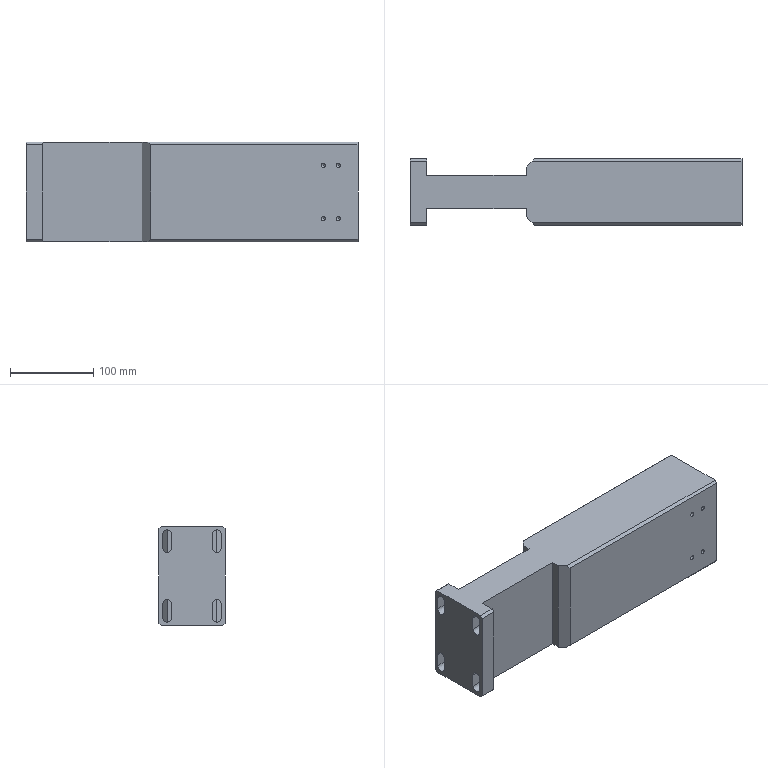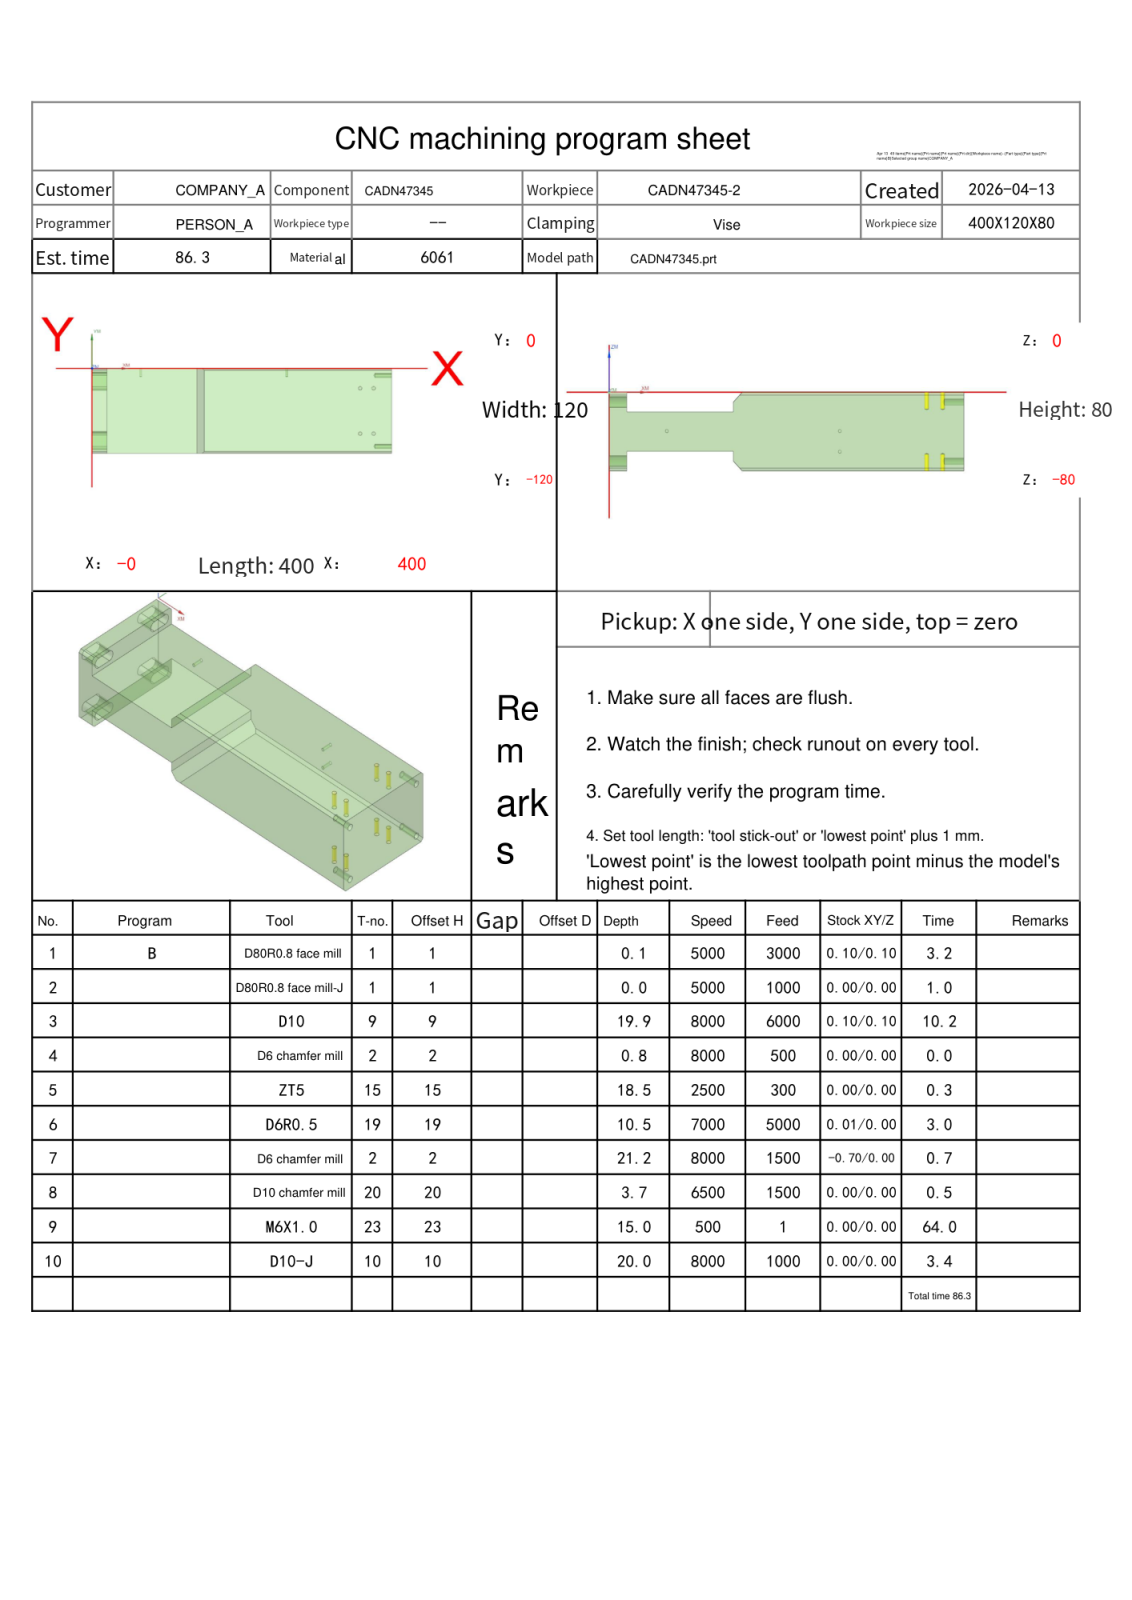NC program | NX | posted by the shop | part box 400 x 80 x 120 mm
Lines 3572 to 4568 of 4568:
N4 T02 M06
(D6 chamfer mill  D=6. R=0. H=02 ce=0.00 di=0.10)
G00 G90 G54 X358. Y-92. M03 S8000
G43 H02 Z20.
M08
G98 G81 X358. Y-92. Z-.8 R1. F500.
X376.
Y-28.
X358.
G80
G00 Z20.
G91 G28 Z0.0
M05
M09
G91 G28 Z0.0
M01
N5 T15 M06
(ZT5 D=5. DR_a=118 H=15)
G00 G90 G54 X358. Y-92. M03 S2500
G43 H15 Z20.
M08
G98 G83 X358. Y-92. Z-18.502 R1. F300. Q3.
X376.
Y-28.
X358.
G80
G00 Z20.
G91 G28 Z0.0
M05
M09
G91 G28 Z0.0
M01
N6 T19 M06
(D6R0.5  D=6. R=0.5 H=19 ce=0.01 di=0.00)
G00 G90 G54 X147.199 Y-123.373 M03 S7000
G43 H19 Z14.8
M08
Z.415
G01 Z-.085 F5000.
Y-118.246
Y-1.754
X147.116 Y-1.668 Z-.17
X147.113 Y-1.725
Y-118.275
X147.116 Y-118.332
X147.032 Y-118.417 Z-.255
X147.028 Y-118.275
Y-1.725
X147.032 Y-1.583
X146.947 Y-1.497 Z-.339
X146.943 Y-1.725
Y-118.275
X146.947 Y-118.503
X146.86 Y-118.588 Z-.424
X146.859 Y-117.278
Y-2.722
X146.86 Y-1.412
X146.776 Y-1.326 Z-.509
X146.774 Y-1.378
Y-118.622
X146.776 Y-118.674
X146.692 Y-118.759 Z-.594
X146.689 Y-118.622
Y-1.378
X146.692 Y-1.241
X146.607 Y-1.156 Z-.679
X146.604 Y-1.378
Y-118.622
X146.607 Y-118.844
X146.521 Y-118.93 Z-.764
X146.519 Y-117.617
Y-2.383
X146.521 Y-1.07
X146.437 Y-.985 Z-.849
X146.434 Y-1.031
Y-118.969
X146.437 Y-119.015
X146.353 Y-119.099 Z-.933
X146.35 Y-118.969
Y-1.031
X146.353 Y-.901
X146.268 Y-.816 Z-1.018
X146.265 Y-1.031
Y-118.969
X146.268 Y-119.184
X146.181 Y-119.269 Z-1.103
X146.18 Y-117.957
Y-2.043
X146.181 Y-.731
X146.097 Y-.646 Z-1.188
X146.095 Y-.684
Y-119.316
X146.097 Y-119.354
X146.013 Y-119.438 Z-1.273
X146.01 Y-119.316
Y-.684
X146.013 Y-.562
X145.929 Y-.477 Z-1.358
X145.925 Y-.684
Y-119.316
X145.929 Y-119.523
X145.842 Y-119.608 Z-1.442
X145.84 Y-118.296
Y-1.704
X145.842 Y-.392
X145.757 Y-.307 Z-1.527
X145.756 Y-.337
Y-119.663
X145.757 Y-119.693
X145.674 Y-119.778 Z-1.612
X145.671 Y-119.663
Y-.337
X145.674 Y-.223
X145.589 Y-.138 Z-1.697
X145.586 Y-.337
Y-119.663
X145.589 Y-119.862
X145.503 Y-119.946 Z-1.782
X145.501 Y-118.635
Y-1.365
X145.503 Y-.054
X145.417 Y.03 Z-1.867
X145.416 Y-1.28
Y-118.72
X145.417 Y-120.03
X145.334 Y-120.114 Z-1.952
X145.331 Y-120.009
Y.009
X145.334 Y.114
X145.25 Y.198 Z-2.036
X145.246 Y.009
Y-120.009
X145.25 Y-120.198
X145.164 Y-120.282 Z-2.121
X145.162 Y-118.975
Y-1.025
X145.164 Y.282
X145.077 Y.366 Z-2.206
Y-.94
Y-119.06
Y-120.366
X144.995 Y-120.45 Z-2.291
X144.992 Y-120.356
Y.356
X144.995 Y.45
X144.911 Y.534 Z-2.376
X144.907 Y.356
Y-120.356
X144.911 Y-120.534
X144.825 Y-120.618 Z-2.461
X144.822 Y-119.314
Y-.686
X144.825 Y.618
X144.737 Y.702 Z-2.546
Y-.601
Y-119.399
Y-120.702
X144.653 Y-120.786 Z-2.63
X144.652 Y-119.484
Y-.516
X144.653 Y.787
X144.571 Y.87 Z-2.715
X144.568 Y.703
Y-120.703
X144.571 Y-120.87
X144.486 Y-120.954 Z-2.8
X144.483 Y-120.703
Y.703
X144.486 Y.954
X144.398 Y1.039 Z-2.885
Y-.261
Y-119.739
Y-121.039
X144.355 Y-121.05 Z-2.927
X144.314 Y-121.061 Z-2.97
X144.313 Y-119.823
Y-.177
X144.314 Y1.061
X144.271 Y1.062 Z-3.012
X144.229 Z-3.055
X144.228 Y-.092
Y-119.908
X144.229 Y-121.063
X144.186 Z-3.097
X144.144 Z-3.14
X144.143 Y-119.993
Y-.007
X144.144 Y1.063
X144.101 Y1.064 Z-3.182
X144.059 Z-3.224
X144.058 Y0.0
Y-120.
X144.059 Y-121.064
X144.016 Y-121.065 Z-3.267
X143.974 Z-3.309
Y-120.
Y0.0
Y1.065
X143.931 Y1.066 Z-3.352
X143.89 Z-3.394
X143.889 Y0.0
Y-120.
X143.89 Y-121.066
X143.846 Y-121.067 Z-3.437
X143.805 Z-3.479
X143.804 Y-120.
Y0.0
X143.805 Y1.067
X143.762 Z-3.521
X143.72 Y1.068 Z-3.564
X143.719 Y0.0
Y-120.
X143.72 Y-121.068
X143.677 Z-3.606
X143.635 Y-121.069 Z-3.649
X143.634 Y-120.
Y0.0
X143.635 Y1.069
X143.592 Z-3.691
X143.55 Y1.07 Z-3.734
X143.549 Y0.0
Y-120.
X143.55 Y-121.07
X143.507 Z-3.776
X143.466 Y-121.071 Z-3.818
X143.465 Y-120.
Y0.0
X143.466 Y1.071
X143.422 Z-3.861
X143.381 Y1.072 Z-3.903
X143.38 Y0.0
Y-120.
X143.381 Y-121.071
X143.337 Y-121.072 Z-3.946
X143.296 Z-3.988
X143.295 Y-120.
Y0.0
X143.296 Y1.072
X143.252 Y1.073 Z-4.031
X143.211 Z-4.073
X143.21 Y0.0
Y-120.
X143.211 Y-121.073
X143.168 Y-121.074 Z-4.115
X143.126 Z-4.158
X143.125 Y-120.
Y0.0
X143.126 Y1.074
X143.083 Y1.075 Z-4.2
X143.042 Z-4.243
X143.04 Y1.05
Y-121.05
X143.042 Y-121.075
X142.998 Z-4.285
X142.957 Y-121.076 Z-4.327
X142.955 Y-121.05
Y1.05
X142.957 Y1.076
X142.913 Z-4.37
X142.872 Y1.077 Z-4.412
X142.871 Y1.05
Y-121.05
X142.872 Y-121.077
X142.828 Z-4.455
X142.789 Z-4.497
X142.788 Y-121.05
Y1.05
X142.789 Y1.077
X142.743 Y1.078 Z-4.54
X142.702 Z-4.582
X142.701 Y1.05
Y-121.05
X142.702 Y-121.078
X142.658 Y-121.079 Z-4.624
X142.617 Z-4.667
X142.616 Y-121.05
Y1.05
X142.617 Y1.079
X142.574 Z-4.709
X142.533 Z-4.752
X142.531 Y1.05
Y-121.05
X142.533 Y-121.08
X142.489 Z-4.794
X142.448 Z-4.837
X142.446 Y-121.05
Y1.05
X142.448 Y1.08
X142.404 Z-4.879
X142.363 Y1.081 Z-4.921
X142.361 Y1.05
Y-121.05
X142.363 Y-121.081
X142.319 Z-4.964
X142.278 Z-5.006
X142.277 Y-121.05
Y1.05
X142.278 Y1.081
X142.234 Y1.082 Z-5.049
X142.193 Z-5.091
X142.192 Y1.05
Y-121.05
X142.193 Y-121.082
X142.149 Z-5.134
X142.108 Z-5.176
X142.107 Y-121.05
Y1.05
X142.108 Y1.082
X142.064 Y1.083 Z-5.218
X142.024 Z-5.261
X142.022 Y1.05
Y-121.05
X142.024 Y-121.083
X141.98 Z-5.303
X141.939 Y-121.084 Z-5.346
X141.937 Y-121.05
Y1.05
X141.939 Y1.084
X141.895 Z-5.388
X141.854 Z-5.431
X141.852 Y1.05
Y-121.05
X141.854 Y-121.084
X141.81 Y-121.085 Z-5.473
X141.769 Z-5.515
X141.767 Y-121.05
Y1.05
X141.769 Y1.085
X141.725 Z-5.558
X141.684 Z-5.6
X141.683 Y1.05
Y-121.05
X141.684 Y-121.085
X141.64 Y-121.086 Z-5.643
X141.6 Z-5.685
X141.598 Y-121.05
Y1.05
X141.599 Y1.086
X141.555 Z-5.728
X141.515 Z-5.77
X141.513 Y1.05
Y-121.05
X141.515 Y-121.086
X141.47 Y-121.087 Z-5.812
X141.43 Z-5.855
X141.428 Y-121.05
Y1.05
X141.43 Y1.087
X141.386 Z-5.897
X141.345 Z-5.94
X141.343 Y1.05
Y-121.05
X141.345 Y-121.087
X141.301 Z-5.982
X141.26 Z-6.025
X141.258 Y-121.05
Y1.05
X141.26 Y1.088
X141.216 Z-6.067
X141.175 Z-6.109
X141.173 Y1.05
Y-121.05
X141.175 Y-121.088
X141.131 Z-6.152
X141.09 Z-6.194
X141.089 Y-121.05
Y1.05
X141.09 Y1.088
X141.046 Z-6.237
X141.006 Z-6.279
X141.004 Y1.05
Y-121.05
X141.006 Y-121.088
X140.961 Z-6.322
X140.921 Z-6.364
X140.919 Y-121.05
Y1.05
X140.921 Y1.088
X140.877 Z-6.406
X140.836 Z-6.449
X140.834 Y1.05
Y-121.05
X140.836 Y-121.088
X140.792 Z-6.491
X140.751 Z-6.534
X140.749 Y-121.05
Y1.05
X140.751 Y1.088
X140.707 Z-6.576
X140.666 Z-6.619
X140.664 Y1.05
Y-121.05
X140.666 Y-121.089
X140.622 Z-6.661
X140.581 Z-6.703
X140.58 Y-120.
Y1.05
X140.581 Y1.089
X140.537 Z-6.746
X140.496 Z-6.788
X140.495 Y1.05
Y-121.05
X140.496 Y-121.089
X140.452 Z-6.831
X140.412 Z-6.873
X140.41 Y-121.05
Y1.05
X140.412 Y1.089
X140.367 Z-6.916
X140.327 Z-6.958
X140.325 Y1.05
Y-121.05
X140.327 Y-121.089
X140.283 Z-7.
X140.242 Z-7.043
X140.24 Y-120.
Y1.05
X140.242 Y1.089
X140.198 Z-7.085
X140.157 Z-7.128
X140.155 Y1.05
Y-121.05
X140.157 Y-121.089
X140.113 Z-7.17
X140.072 Z-7.212
X140.07 Y-121.05
Y1.05
X140.072 Y1.089
X140.028 Z-7.255
X139.987 Z-7.297
X139.986 Y1.05
Y-121.05
X139.987 Y-121.089
X139.943 Z-7.34
X139.903 Z-7.382
X139.901 Y-121.05
Y1.05
X139.903 Y1.089
X139.858 Z-7.425
X139.818 Z-7.467
X139.816 Y1.05
Y-121.05
X139.818 Y-121.089
X139.773 Z-7.509
X139.733 Z-7.552
X139.731 Y-121.05
Y1.05
X139.733 Y1.089
X139.689 Z-7.594
X139.648 Y1.088 Z-7.637
X139.646 Y1.05
Y-121.05
X139.648 Y-121.088
X139.604 Z-7.679
X139.563 Z-7.722
X139.561 Y-121.05
Y1.05
X139.563 Y1.088
X139.519 Z-7.764
X139.478 Z-7.806
X139.476 Y1.05
Y-121.05
X139.478 Y-121.088
X139.434 Z-7.849
X139.393 Y-121.087 Z-7.891
X139.392 Y-121.05
Y1.05
X139.393 Y1.088
X139.349 Y1.087 Z-7.934
X139.309 Z-7.976
X139.307 Y1.05
Y-121.05
X139.309 Y-121.087
X139.264 Z-8.019
X139.224 Z-8.061
X139.222 Y-121.05
Y1.05
X139.224 Y1.087
X139.179 Z-8.103
X139.139 Z-8.146
X139.137 Y1.05
Y-121.05
X139.139 Y-121.086
X139.095 Z-8.188
X139.054 Z-8.231
X139.052 Y-121.05
Y1.05
X139.054 Y1.086
X139.01 Z-8.273
X138.969 Z-8.316
X138.967 Y1.05
Y-121.05
X138.969 Y-121.086
X138.925 Z-8.358
X138.884 Z-8.4
X138.882 Y-121.05
Y1.05
X138.884 Y1.086
X138.84 Z-8.443
X138.799 Y1.085 Z-8.485
X138.798 Y1.05
Y-121.05
X138.799 Y-121.085
X138.755 Z-8.528
X138.714 Z-8.57
X138.713 Y-121.05
Y1.05
X138.714 Y1.085
X138.67 Z-8.613
X138.63 Z-8.655
X138.628 Y1.05
Y-121.05
X138.63 Y-121.085
X138.585 Y-121.084 Z-8.697
X138.545 Z-8.74
X138.543 Y-121.05
Y1.05
X138.545 Y1.084
X138.501 Z-8.782
X138.46 Z-8.825
X138.458 Y1.05
Y-121.05
X138.46 Y-121.084
X138.416 Z-8.867
X138.375 Y-121.083 Z-8.91
X138.373 Y-121.05
Y1.05
X138.375 Y1.083
X138.331 Z-8.952
X138.29 Z-8.994
X138.288 Y1.05
Y-121.05
X138.29 Y-121.083
X138.246 Y-121.082 Z-9.037
X138.205 Z-9.079
X138.204 Y-121.05
Y1.05
X138.205 Y1.082
X138.161 Z-9.122
X138.12 Y1.081 Z-9.164
X138.119 Y1.05
Y-121.05
X138.12 Y-121.082
X138.076 Y-121.081 Z-9.207
X138.035 Z-9.249
X138.034 Y-121.05
Y1.05
X138.035 Y1.081
X137.992 Z-9.291
X137.951 Y1.08 Z-9.334
X137.949 Y1.05
Y-121.05
X137.951 Y-121.08
X137.907 Z-9.376
X137.866 Z-9.419
X137.864 Y-121.05
Y1.05
X137.866 Y1.08
X137.822 Y1.079 Z-9.461
X137.781 Z-9.504
X137.779 Y1.05
Y-121.05
X137.781 Y-121.079
X137.737 Z-9.546
X137.696 Z-9.588
X137.695 Y-121.05
Y1.05
X137.696 Y1.079
X137.652 Y1.078 Z-9.631
X137.611 Z-9.673
X137.61 Y1.05
Y-121.05
X137.611 Y-121.078
X137.567 Z-9.716
X137.526 Z-9.758
X137.525 Y-121.05
Y1.05
X137.526 Y1.077
X137.482 Z-9.801
X137.441 Z-9.843
X137.44 Y1.05
Y-121.05
X137.441 Y-121.077
X137.398 Z-9.885
X137.356 Y-121.076 Z-9.928
X137.355 Y-121.05
Y1.05
X137.356 Y1.076
X137.313 Z-9.97
X137.272 Z-10.013
X137.27 Y1.05
Y-121.05
X137.272 Y-121.076
X137.228 Y-121.075 Z-10.055
X137.187 Z-10.097
X137.185 Y-121.05
Y1.05
X137.187 Y1.075
X137.143 Z-10.14
X137.102 Z-10.182
Y-121.075
X137.061 Y-121.074 Z-10.222
X137.022 Z-10.262
Y1.074
X136.981 Z-10.301
X136.943 Z-10.341
Y-121.074
X136.902 Y-121.073 Z-10.381
X136.864 Z-10.421
Y1.073
X136.823 Z-10.46
X136.784 Z-10.5
Y-121.073
G00 Z14.8
G91 G28 Z0.0
M05
M09
G91 G28 Z0.0
M01
N7 T02 M06
(D6 chamfer mill  D=6. R=0. H=02 ce=0.00 di=0.00)
G00 G90 G54 X20.99 Y-2.208 M03 S6500
G43 H02 Z20.
M08
Z.13
G01 Z-1.2 F1500.
G03 X20.915 Y-2.548 I1.907 J-.601
G01 X20.905 Y-2.602
X20.928 Y-2.651
X20.966 Y-2.741
X21. Y-3.
Y-117.
X20.966 Y-117.259
X20.928 Y-117.349
X20.905 Y-117.398
X20.915 Y-117.452
G03 X20.99 Y-117.792 I1.983 J.261
G01 Z.13
G00 Z10.
X-.99
Z.13
G01 Z-1.2
G03 X-.915 Y-117.452 I-1.907 J.601
G01 X-.905 Y-117.398
X-.928 Y-117.349
X-.966 Y-117.259
X-1. Y-117.
Y-60.
Y-3.
X-.966 Y-2.741
X-.928 Y-2.651
X-.905 Y-2.602
X-.915 Y-2.548
G03 X-.99 Y-2.208 I-1.983 J-.261
G01 Z.13
G00 Z10.
X400.99
Z.13
G01 Z-1.2
G03 X400.915 Y-2.548 I1.907 J-.601
G01 X400.905 Y-2.602
X400.928 Y-2.651
X400.966 Y-2.741
X401. Y-3.
Y-117.
X400.966 Y-117.259
X400.928 Y-117.349
X400.905 Y-117.398
X400.915 Y-117.452
G03 X400.99 Y-117.792 I1.983 J.261
G01 Z.13
G00 Z10.
X357.593 Y-29.315
Z.284
G01 Z-1.2
G03 X357.898 Y-29.484 I1.118 J1.658
G01 X357.946 Y-29.509
X358. Y-29.5
G03 X359.5 Y-28. I0.0 J1.5
X358. Y-26.5 I-1.5 J0.0
X356.5 Y-28. I0.0 J-1.5
X358. Y-29.5 I1.5 J0.0
G01 X358.054 Y-29.509
X358.102 Y-29.484
G03 X358.407 Y-29.315 I-.813 J1.827
G01 Z.284
G00 Z10.
X375.593
Z.284
G01 Z-1.2
G03 X375.898 Y-29.484 I1.118 J1.658
G01 X375.946 Y-29.509
X376. Y-29.5
G03 X377.5 Y-28. I0.0 J1.5
X376. Y-26.5 I-1.5 J0.0
X374.5 Y-28. I0.0 J-1.5
X376. Y-29.5 I1.5 J0.0
G01 X376.054 Y-29.509
X376.102 Y-29.484
G03 X376.407 Y-29.315 I-.813 J1.827
G01 Z.284
G00 Z10.
X375.593 Y-93.315
Z.284
G01 Z-1.2
G03 X375.898 Y-93.484 I1.118 J1.658
G01 X375.946 Y-93.509
X376. Y-93.5
G03 X377.5 Y-92. I0.0 J1.5
X376. Y-90.5 I-1.5 J0.0
X374.5 Y-92. I0.0 J-1.5
X376. Y-93.5 I1.5 J0.0
G01 X376.054 Y-93.509
X376.102 Y-93.484
G03 X376.407 Y-93.315 I-.813 J1.827
G01 Z.284
G00 Z10.
X357.593
Z.284
G01 Z-1.2
G03 X357.898 Y-93.484 I1.118 J1.658
G01 X357.946 Y-93.509
X358. Y-93.5
G03 X359.5 Y-92. I0.0 J1.5
X358. Y-90.5 I-1.5 J0.0
X356.5 Y-92. I0.0 J-1.5
X358. Y-93.5 I1.5 J0.0
G01 X358.054 Y-93.509
X358.102 Y-93.484
G03 X358.407 Y-93.315 I-.813 J1.827
G01 Z.284
G00 Z10.
X136.981 Y-121.068
Z-11.096
G01 Z-21.2
X136.895 Y-121.008
X136.865 Y-121.
X23.135
X23.105 Y-121.008
X23.019 Y-121.068
Z-3.291
G00 Z10.
Y1.068
Z-3.291
G01 Z-21.2
X23.105 Y1.008
X23.135 Y1.
X136.865
X136.895 Y1.008
X136.981 Y1.068
Z-11.096
G00 Z20.
G00 G90 X357.13 Y-92.232 M03 S8000
Z20.
Z-.8
G01 Z-1.3 F600.
X356.5 Y-92.4
G03 X358. Y-93.9 I1.5 J0.0
X359.9 Y-92. I0.0 J1.9
X358. Y-90.1 I-1.9 J0.0
X356.1 Y-92. I0.0 J-1.9
X358. Y-93.9 I1.9 J0.0
X359.5 Y-92.4 I0.0 J1.5
G01 X358.87 Y-92.232
Z-.8
G00 Z20.
X375.13
Z-.8
G01 Z-1.3
X374.5 Y-92.4
G03 X376. Y-93.9 I1.5 J0.0
X377.9 Y-92. I0.0 J1.9
X376. Y-90.1 I-1.9 J0.0
X374.1 Y-92. I0.0 J-1.9
X376. Y-93.9 I1.9 J0.0
X377.5 Y-92.4 I0.0 J1.5
G01 X376.87 Y-92.232
Z-.8
G00 Z20.
X375.13 Y-28.232
Z-.8
G01 Z-1.3
X374.5 Y-28.4
G03 X376. Y-29.9 I1.5 J0.0
X377.9 Y-28. I0.0 J1.9
X376. Y-26.1 I-1.9 J0.0
X374.1 Y-28. I0.0 J-1.9
X376. Y-29.9 I1.9 J0.0
X377.5 Y-28.4 I0.0 J1.5
G01 X376.87 Y-28.232
Z-.8
G00 Z20.
X357.13
Z-.8
G01 Z-1.3
X356.5 Y-28.4
G03 X358. Y-29.9 I1.5 J0.0
X359.9 Y-28. I0.0 J1.9
X358. Y-26.1 I-1.9 J0.0
X356.1 Y-28. I0.0 J-1.9
X358. Y-29.9 I1.9 J0.0
X359.5 Y-28.4 I0.0 J1.5
G01 X358.87 Y-28.232
Z-.8
G00 Z20.
G91 G28 Z0.0
M05
M09
G91 G28 Z0.0
M01
N8 T20 M06
(D10 chamfer mill  D=10. R=0. H=20 ce=0.00 di=0.00)
G00 G90 G54 X25.7 Y-121.028 M03 S6500
G43 H20 Z20.
M08
Z-2.2
G01 Z-3.7 F1500.
G03 X24.603 Y-120.7 I-1.097 J-1.672
G01 X-4.603
G03 X-5.7 Y-121.028 I0.0 J-2.
G01 Z-2.2
G00 Z20.
Y1.028
Z-2.2
G01 Z-3.7
G03 X-4.603 Y.7 I1.097 J1.672
G01 X24.603
G03 X25.7 Y1.028 I0.0 J2.
G01 Z-2.2
G00 Z20.
X140.397 Y2.7
Z-2.2
G01 Z-3.7
G03 X142.397 Y.7 I2. J0.0
G01 X404.603
G03 X405.7 Y1.028 I0.0 J2.
G01 Z-2.2
G00 Z20.
Y-121.028
Z-2.2
G01 Z-3.7
G03 X404.603 Y-120.7 I-1.097 J-1.672
G01 X142.397
G03 X140.397 Y-122.7 I0.0 J-2.
G01 Z-2.2
G00 Z20.
G91 G28 Z0.0
M05
M09
G91 G28 Z0.0
M01
N9 T23 M06
(M6X1.0 D=5. DR_a=180 H=23)
G00 G90 G54 X358. Y-92. M03 S500
G43 H23 Z20.
M08
G95
G98 G84 X358. Y-92. Z-15. R1. F1. Q3.
X376.
Y-28.
X358.
G80
G94
G00 Z20.
G91 G28 Z0.0
M05
M09
G91 G28 Z0.0
M01
N10 T10 M06
(D10-J  D=10. R=0. H=10 ce=0.40 di=0.00)
G00 G90 G54 X27.401 Y-127. M03 S8000
G43 H10 Z14.8
M08
Z-18.5
G01 Z-20. F1000.
Y-123.
G03 X25.401 Y-125. I0.0 J-2.
G01 Y4.1
G02 X26.301 Y5. I.9 J0.0
G01 X29.365
G02 X30.365 Y4. I0.0 J-1.
G01 Y-124.1
G03 X31.265 Y-125. I.9 J0.0
G01 X34.328
G03 X35.328 Y-124. I0.0 J1.
G01 Y4.1
G02 X36.228 Y5. I.9 J0.0
G01 X39.292
G02 X40.292 Y4. I0.0 J-1.
G01 Y-124.1
G03 X41.192 Y-125. I.9 J0.0
G01 X44.255
G03 X45.255 Y-124. I0.0 J1.
G01 Y4.1
G02 X46.155 Y5. I.9 J0.0
G01 X49.219
G02 X50.219 Y4. I0.0 J-1.
G01 Y-124.1
G03 X51.119 Y-125. I.9 J0.0
G01 X54.183
G03 X55.183 Y-124. I0.0 J1.
G01 Y4.1
G02 X56.083 Y5. I.9 J0.0
G01 X59.146
G02 X60.146 Y4. I0.0 J-1.
G01 Y-124.1
G03 X61.046 Y-125. I.9 J0.0
G01 X64.11
G03 X65.11 Y-124. I0.0 J1.
G01 Y4.1
G02 X66.01 Y5. I.9 J0.0
G01 X69.073
G02 X70.073 Y4. I0.0 J-1.
G01 Y-124.1
G03 X70.973 Y-125. I.9 J0.0
G01 X74.037
G03 X75.037 Y-124. I0.0 J1.
G01 Y4.1
G02 X75.937 Y5. I.9 J0.0
G01 X79.
G02 X80. Y4. I0.0 J-1.
G01 Y-124.1
G03 X80.9 Y-125. I.9 J0.0
G01 X83.964
G03 X84.964 Y-124. I0.0 J1.
G01 Y4.1
G02 X85.864 Y5. I.9 J0.0
G01 X88.928
G02 X89.928 Y4. I0.0 J-1.
G01 Y-124.1
G03 X90.828 Y-125. I.9 J0.0
G01 X93.891
G03 X94.891 Y-124. I0.0 J1.
G01 Y4.1
G02 X95.791 Y5. I.9 J0.0
G01 X98.855
G02 X99.855 Y4. I0.0 J-1.
G01 Y-124.1
G03 X100.755 Y-125. I.9 J0.0
G01 X103.818
G03 X104.818 Y-124. I0.0 J1.
G01 Y4.1
G02 X105.718 Y5. I.9 J0.0
G01 X108.782
G02 X109.782 Y4. I0.0 J-1.
G01 Y-124.1
G03 X110.682 Y-125. I.9 J0.0
G01 X113.746
G03 X114.746 Y-124. I0.0 J1.
G01 Y4.1
G02 X115.646 Y5. I.9 J0.0
G01 X118.709
G02 X119.709 Y4. I0.0 J-1.
G01 Y-124.1
G03 X120.609 Y-125. I.9 J0.0
G01 X123.673
G03 X124.673 Y-124. I0.0 J1.
G01 Y4.1
G02 X125.573 Y5. I.9 J0.0
G01 X128.636
G02 X129.636 Y4. I0.0 J-1.
G01 Y-124.1
G03 X130.536 Y-125. I.9 J0.0
G01 X133.6
G03 X134.6 Y-124. I0.0 J1.
G01 Y5.
G03 X132.6 Y7. I-2. J0.0
G01 Z-18.5
G00 Z14.8
G00 G90 X132.801 Y-127. M03 S8000
Z14.8
Z-19.
G01 Z-20. F1000.
G41 D10
X133.001
G03 X135. Y-125. I-.001 J2.
G01 Y5.
G03 X133.001 Y7. I-2. J0.0
G01 G40 X132.801
Z-19.
G00 X27.199
G01 Z-20.
G41 D10
X26.999
G03 X25. Y5. I.001 J-2.
G01 Y-125.
G03 X26.999 Y-127. I2. J0.0
G01 G40 X27.199
Z-19.
G00 Z14.8
M05
M09
G91 G28 Z0.0
G91 G28 Y0.0
M30
%